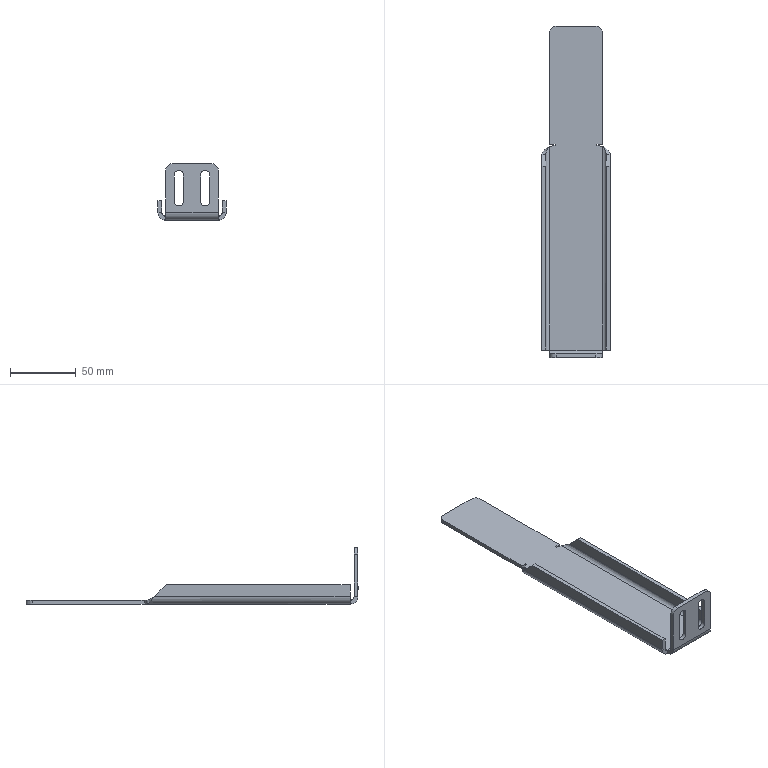Part | SolidWorks | features SM3dBend 2, FlatPattern 1, SMBaseFlange 1, SheetMetal 1 | 1 solid | 54 faces | box 52 x 253 x 42.931 mm | volume 47951 mm3 | plane 36 | cylinder 14 | spline 4 | commonest cylinder face diameters 7 x4 10 x4 6 x3 12 x3